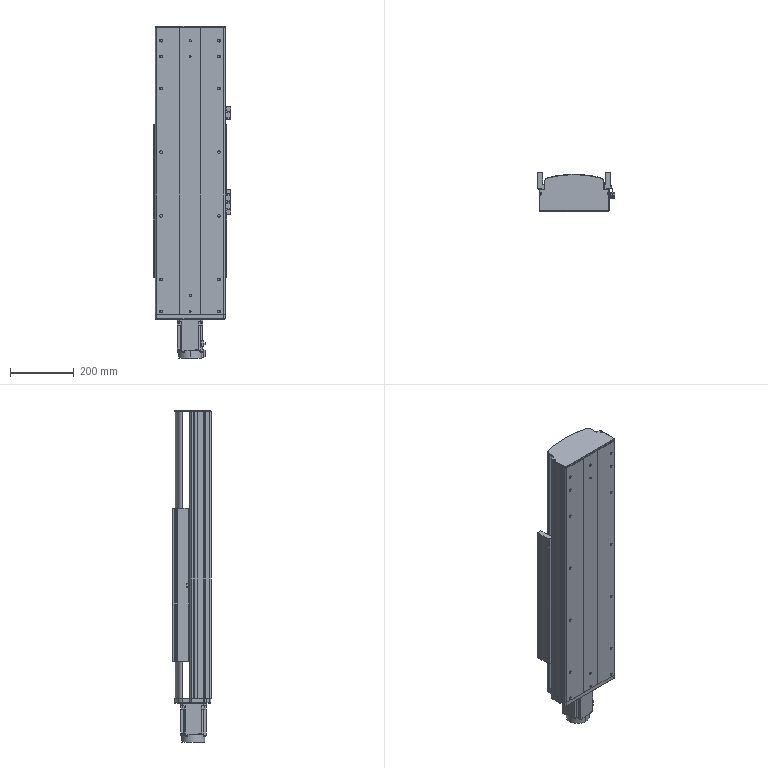Part | SolidWorks | features AEMSimFeature 1 | 30 solids | 1317 faces | box 242 x 122 x 1042 mm | volume 13192618 mm3 | plane 687 | cylinder 492 | cone 82 | torus 56 | commonest cylinder face diameters 0.5 x36 5.5 x36 2.5 x32 1 x30 3 x28 8.6 x28